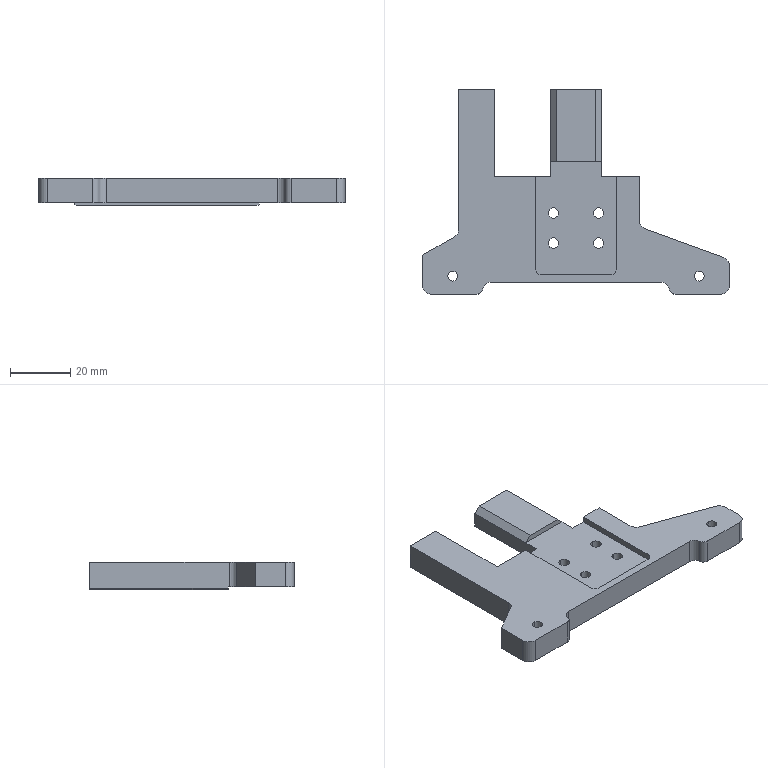Part | 1 solid | 80 faces | box 102 x 68 x 9.2 mm | volume 28644 mm3 | plane 40 | cylinder 39 | cone 1 | commonest cylinder face diameters 6 x15 3.5 x8 4 x8 3.3 x4 2.5 x2 5 x2